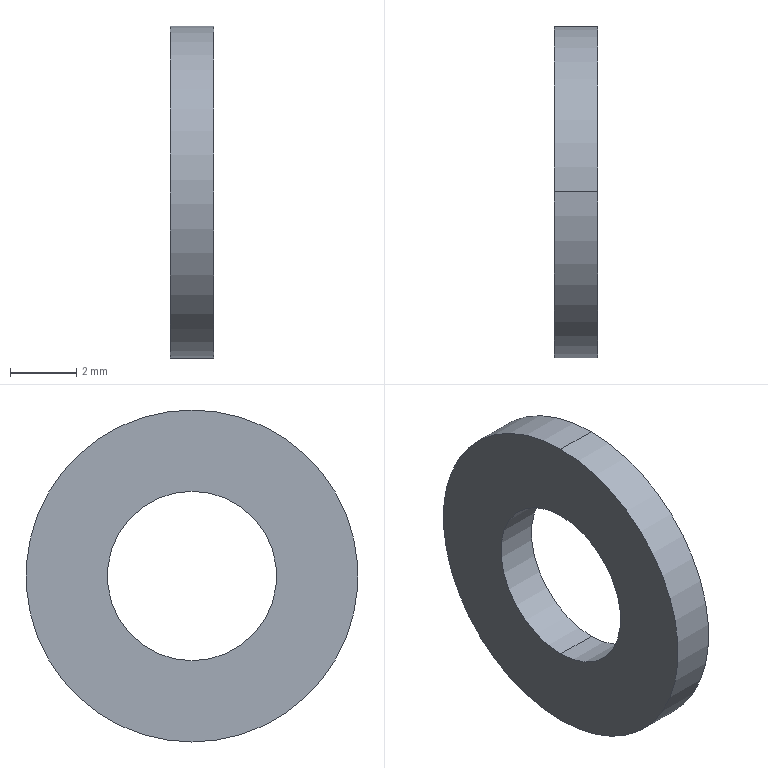Part | STEP file | 0245_Z_041_HCBST5-16_2 | 1 solid | 6 faces | box 1.3 x 10 x 10 mm | volume 75.545 mm3 | cylinder 4 | plane 2 | commonest cylinder face diameters 5.1 x2 10 x2
STEP:
#1=CARTESIAN_POINT('',(0.,0.,0.));
#2=DIRECTION('',(0.,0.,1.));
#3=DIRECTION('',(1.,0.,0.));
#4=AXIS2_PLACEMENT_3D('',#1,#2,#3);
#5=CARTESIAN_POINT('',(4.9,0.,2.55));
#6=VERTEX_POINT('',#5);
#7=CARTESIAN_POINT('',(3.6,0.,2.55));
#8=VERTEX_POINT('',#7);
#9=CARTESIAN_POINT('',(3.6,0.,2.55));
#10=DIRECTION('',(-1.,0.,0.));
#11=VECTOR('',#10,1.);
#12=LINE('',#9,#11);
#13=CARTESIAN_POINT('',(3.6,0.,0.));
#14=DIRECTION('',(-1.,0.,0.));
#15=DIRECTION('',(0.,0.,1.));
#16=AXIS2_PLACEMENT_3D('',#13,#14,#15);
#17=CYLINDRICAL_SURFACE('',#16,2.55);
#18=CARTESIAN_POINT('',(6.283,0.));
#19=DIRECTION('',(0.,1.));
#20=VECTOR('',#19,1.);
#21=LINE('',#18,#20);
#22=(GEOMETRIC_REPRESENTATION_CONTEXT(2)PARAMETRIC_REPRESENTATION_CONTEXT()REPRESENTATION_CONTEXT('',''));
#23=DEFINITIONAL_REPRESENTATION('',(#21),#22);
#24=PCURVE('',#17,#23);
#25=CARTESIAN_POINT('',(3.6,0.,0.));
#26=DIRECTION('',(-1.,0.,0.));
#27=DIRECTION('',(0.,0.,1.));
#28=AXIS2_PLACEMENT_3D('',#25,#26,#27);
#29=CYLINDRICAL_SURFACE('',#28,2.55);
#30=CARTESIAN_POINT('',(0.,0.));
#31=DIRECTION('',(0.,1.));
#32=VECTOR('',#31,1.);
#33=LINE('',#30,#32);
#34=(GEOMETRIC_REPRESENTATION_CONTEXT(2)PARAMETRIC_REPRESENTATION_CONTEXT()REPRESENTATION_CONTEXT('',''));
#35=DEFINITIONAL_REPRESENTATION('',(#33),#34);
#36=PCURVE('',#29,#35);
#37=SURFACE_CURVE('',#12,(#24,#36),.PCURVE_S1.);
#38=EDGE_CURVE('',#6,#8,#37,.T.);
#39=ORIENTED_EDGE('',*,*,#38,.T.);
#40=CARTESIAN_POINT('',(3.6,0.,-2.55));
#41=VERTEX_POINT('',#40);
#42=CARTESIAN_POINT('',(3.6,0.,0.));
#43=DIRECTION('',(1.,0.,0.));
#44=DIRECTION('',(0.,0.,1.));
#45=AXIS2_PLACEMENT_3D('',#42,#43,#44);
#46=CIRCLE('',#45,2.55);
#47=CARTESIAN_POINT('',(6.283,0.));
#48=DIRECTION('',(-1.,0.));
#49=VECTOR('',#48,1.);
#50=LINE('',#47,#49);
#51=(GEOMETRIC_REPRESENTATION_CONTEXT(2)PARAMETRIC_REPRESENTATION_CONTEXT()REPRESENTATION_CONTEXT('',''));
#52=DEFINITIONAL_REPRESENTATION('',(#50),#51);
#53=PCURVE('',#17,#52);
#54=CARTESIAN_POINT('',(3.6,0.,0.));
#55=DIRECTION('',(-1.,0.,0.));
#56=DIRECTION('',(0.,0.,1.));
#57=AXIS2_PLACEMENT_3D('',#54,#55,#56);
#58=PLANE('',#57);
#59=CARTESIAN_POINT('',(2.55,0.));
#60=CARTESIAN_POINT('',(2.55,-4.417));
#61=CARTESIAN_POINT('',(-1.275,-2.208));
#62=CARTESIAN_POINT('',(-5.1,0.));
#63=CARTESIAN_POINT('',(-1.275,2.208));
#64=CARTESIAN_POINT('',(2.55,4.417));
#65=CARTESIAN_POINT('',(2.55,0.));
#66=(BOUNDED_CURVE()B_SPLINE_CURVE(2,(#59,#60,#61,#62,#63,#64,#65),.UNSPECIFIED.,.T.,.F.)B_SPLINE_CURVE_WITH_KNOTS((1,2,2,2,2,1),(-2.094,0.,2.094,4.189,6.283,8.378),.UNSPECIFIED.)CURVE()GEOMETRIC_REPRESENTATION_ITEM()RATIONAL_B_SPLINE_CURVE((1.,0.5,1.,0.5,1.,0.5,1.))REPRESENTATION_ITEM(''));
#67=(GEOMETRIC_REPRESENTATION_CONTEXT(2)PARAMETRIC_REPRESENTATION_CONTEXT()REPRESENTATION_CONTEXT('',''));
#68=DEFINITIONAL_REPRESENTATION('',(#66),#67);
#69=PCURVE('',#58,#68);
#70=SURFACE_CURVE('',#46,(#53,#69),.PCURVE_S1.);
#71=EDGE_CURVE('',#8,#41,#70,.T.);
#72=ORIENTED_EDGE('',*,*,#71,.T.);
#73=CARTESIAN_POINT('',(4.9,0.,-2.55));
#74=VERTEX_POINT('',#73);
#75=CARTESIAN_POINT('',(3.6,0.,-2.55));
#76=DIRECTION('',(-1.,0.,0.));
#77=VECTOR('',#76,1.);
#78=LINE('',#75,#77);
#79=CARTESIAN_POINT('',(3.142,0.));
#80=DIRECTION('',(0.,1.));
#81=VECTOR('',#80,1.);
#82=LINE('',#79,#81);
#83=(GEOMETRIC_REPRESENTATION_CONTEXT(2)PARAMETRIC_REPRESENTATION_CONTEXT()REPRESENTATION_CONTEXT('',''));
#84=DEFINITIONAL_REPRESENTATION('',(#82),#83);
#85=PCURVE('',#17,#84);
#86=CARTESIAN_POINT('',(3.142,0.));
#87=DIRECTION('',(0.,1.));
#88=VECTOR('',#87,1.);
#89=LINE('',#86,#88);
#90=(GEOMETRIC_REPRESENTATION_CONTEXT(2)PARAMETRIC_REPRESENTATION_CONTEXT()REPRESENTATION_CONTEXT('',''));
#91=DEFINITIONAL_REPRESENTATION('',(#89),#90);
#92=PCURVE('',#29,#91);
#93=SURFACE_CURVE('',#78,(#85,#92),.PCURVE_S1.);
#94=EDGE_CURVE('',#74,#41,#93,.T.);
#95=ORIENTED_EDGE('',*,*,#94,.F.);
#96=CARTESIAN_POINT('',(4.9,0.,0.));
#97=DIRECTION('',(1.,0.,0.));
#98=DIRECTION('',(0.,0.,1.));
#99=AXIS2_PLACEMENT_3D('',#96,#97,#98);
#100=CIRCLE('',#99,2.55);
#101=CARTESIAN_POINT('',(6.283,-1.3));
#102=DIRECTION('',(-1.,0.));
#103=VECTOR('',#102,1.);
#104=LINE('',#101,#103);
#105=(GEOMETRIC_REPRESENTATION_CONTEXT(2)PARAMETRIC_REPRESENTATION_CONTEXT()REPRESENTATION_CONTEXT('',''));
#106=DEFINITIONAL_REPRESENTATION('',(#104),#105);
#107=PCURVE('',#17,#106);
#108=CARTESIAN_POINT('',(4.9,0.,0.));
#109=DIRECTION('',(-1.,0.,0.));
#110=DIRECTION('',(0.,0.,1.));
#111=AXIS2_PLACEMENT_3D('',#108,#109,#110);
#112=PLANE('',#111);
#113=CARTESIAN_POINT('',(2.55,0.));
#114=CARTESIAN_POINT('',(2.55,-4.417));
#115=CARTESIAN_POINT('',(-1.275,-2.208));
#116=CARTESIAN_POINT('',(-5.1,0.));
#117=CARTESIAN_POINT('',(-1.275,2.208));
#118=CARTESIAN_POINT('',(2.55,4.417));
#119=CARTESIAN_POINT('',(2.55,0.));
#120=(BOUNDED_CURVE()B_SPLINE_CURVE(2,(#113,#114,#115,#116,#117,#118,#119),.UNSPECIFIED.,.T.,.F.)B_SPLINE_CURVE_WITH_KNOTS((1,2,2,2,2,1),(-2.094,0.,2.094,4.189,6.283,8.378),.UNSPECIFIED.)CURVE()GEOMETRIC_REPRESENTATION_ITEM()RATIONAL_B_SPLINE_CURVE((1.,0.5,1.,0.5,1.,0.5,1.))REPRESENTATION_ITEM(''));
#121=(GEOMETRIC_REPRESENTATION_CONTEXT(2)PARAMETRIC_REPRESENTATION_CONTEXT()REPRESENTATION_CONTEXT('',''));
#122=DEFINITIONAL_REPRESENTATION('',(#120),#121);
#123=PCURVE('',#112,#122);
#124=SURFACE_CURVE('',#100,(#107,#123),.PCURVE_S1.);
#125=EDGE_CURVE('',#6,#74,#124,.T.);
#126=ORIENTED_EDGE('',*,*,#125,.F.);
#127=EDGE_LOOP('',(#39,#72,#95,#126));
#128=FACE_BOUND('',#127,.F.);
#129=ADVANCED_FACE('',(#128),#17,.F.);
#130=CARTESIAN_POINT('',(4.9,0.,5.));
#131=VERTEX_POINT('',#130);
#132=CARTESIAN_POINT('',(4.9,0.,-5.));
#133=VERTEX_POINT('',#132);
#134=CARTESIAN_POINT('',(4.9,0.,0.));
#135=DIRECTION('',(-1.,0.,0.));
#136=DIRECTION('',(0.,0.,1.));
#137=AXIS2_PLACEMENT_3D('',#134,#135,#136);
#138=CIRCLE('',#137,5.);
#139=CARTESIAN_POINT('',(3.6,0.,0.));
#140=DIRECTION('',(-1.,0.,0.));
#141=DIRECTION('',(0.,0.,1.));
#142=AXIS2_PLACEMENT_3D('',#139,#140,#141);
#143=CYLINDRICAL_SURFACE('',#142,5.);
#144=CARTESIAN_POINT('',(0.,-1.3));
#145=DIRECTION('',(1.,0.));
#146=VECTOR('',#145,1.);
#147=LINE('',#144,#146);
#148=(GEOMETRIC_REPRESENTATION_CONTEXT(2)PARAMETRIC_REPRESENTATION_CONTEXT()REPRESENTATION_CONTEXT('',''));
#149=DEFINITIONAL_REPRESENTATION('',(#147),#148);
#150=PCURVE('',#143,#149);
#151=CARTESIAN_POINT('',(0.,0.));
#152=DIRECTION('',(1.,0.));
#153=AXIS2_PLACEMENT_2D('',#151,#152);
#154=CIRCLE('',#153,5.);
#155=(GEOMETRIC_REPRESENTATION_CONTEXT(2)PARAMETRIC_REPRESENTATION_CONTEXT()REPRESENTATION_CONTEXT('',''));
#156=DEFINITIONAL_REPRESENTATION('',(#154),#155);
#157=PCURVE('',#112,#156);
#158=SURFACE_CURVE('',#138,(#150,#157),.PCURVE_S1.);
#159=EDGE_CURVE('',#131,#133,#158,.T.);
#160=ORIENTED_EDGE('',*,*,#159,.T.);
#161=CARTESIAN_POINT('',(3.6,0.,-5.));
#162=VERTEX_POINT('',#161);
#163=CARTESIAN_POINT('',(3.6,0.,-5.));
#164=DIRECTION('',(-1.,0.,0.));
#165=VECTOR('',#164,1.);
#166=LINE('',#163,#165);
#167=CARTESIAN_POINT('',(3.142,0.));
#168=DIRECTION('',(0.,1.));
#169=VECTOR('',#168,1.);
#170=LINE('',#167,#169);
#171=(GEOMETRIC_REPRESENTATION_CONTEXT(2)PARAMETRIC_REPRESENTATION_CONTEXT()REPRESENTATION_CONTEXT('',''));
#172=DEFINITIONAL_REPRESENTATION('',(#170),#171);
#173=PCURVE('',#143,#172);
#174=CARTESIAN_POINT('',(3.6,0.,0.));
#175=DIRECTION('',(-1.,0.,0.));
#176=DIRECTION('',(0.,0.,1.));
#177=AXIS2_PLACEMENT_3D('',#174,#175,#176);
#178=CYLINDRICAL_SURFACE('',#177,5.);
#179=CARTESIAN_POINT('',(3.142,0.));
#180=DIRECTION('',(0.,1.));
#181=VECTOR('',#180,1.);
#182=LINE('',#179,#181);
#183=(GEOMETRIC_REPRESENTATION_CONTEXT(2)PARAMETRIC_REPRESENTATION_CONTEXT()REPRESENTATION_CONTEXT('',''));
#184=DEFINITIONAL_REPRESENTATION('',(#182),#183);
#185=PCURVE('',#178,#184);
#186=SURFACE_CURVE('',#166,(#173,#185),.PCURVE_S1.);
#187=EDGE_CURVE('',#133,#162,#186,.T.);
#188=ORIENTED_EDGE('',*,*,#187,.T.);
#189=CARTESIAN_POINT('',(3.6,0.,5.));
#190=VERTEX_POINT('',#189);
#191=CARTESIAN_POINT('',(3.6,0.,0.));
#192=DIRECTION('',(1.,0.,0.));
#193=DIRECTION('',(0.,0.,1.));
#194=AXIS2_PLACEMENT_3D('',#191,#192,#193);
#195=CIRCLE('',#194,5.);
#196=CARTESIAN_POINT('',(6.283,0.));
#197=DIRECTION('',(-1.,0.));
#198=VECTOR('',#197,1.);
#199=LINE('',#196,#198);
#200=(GEOMETRIC_REPRESENTATION_CONTEXT(2)PARAMETRIC_REPRESENTATION_CONTEXT()REPRESENTATION_CONTEXT('',''));
#201=DEFINITIONAL_REPRESENTATION('',(#199),#200);
#202=PCURVE('',#143,#201);
#203=CARTESIAN_POINT('',(5.,0.));
#204=CARTESIAN_POINT('',(5.,-8.66));
#205=CARTESIAN_POINT('',(-2.5,-4.33));
#206=CARTESIAN_POINT('',(-10.,0.));
#207=CARTESIAN_POINT('',(-2.5,4.33));
#208=CARTESIAN_POINT('',(5.,8.66));
#209=CARTESIAN_POINT('',(5.,0.));
#210=(BOUNDED_CURVE()B_SPLINE_CURVE(2,(#203,#204,#205,#206,#207,#208,#209),.UNSPECIFIED.,.T.,.F.)B_SPLINE_CURVE_WITH_KNOTS((1,2,2,2,2,1),(-2.094,0.,2.094,4.189,6.283,8.378),.UNSPECIFIED.)CURVE()GEOMETRIC_REPRESENTATION_ITEM()RATIONAL_B_SPLINE_CURVE((1.,0.5,1.,0.5,1.,0.5,1.))REPRESENTATION_ITEM(''));
#211=(GEOMETRIC_REPRESENTATION_CONTEXT(2)PARAMETRIC_REPRESENTATION_CONTEXT()REPRESENTATION_CONTEXT('',''));
#212=DEFINITIONAL_REPRESENTATION('',(#210),#211);
#213=PCURVE('',#58,#212);
#214=SURFACE_CURVE('',#195,(#202,#213),.PCURVE_S1.);
#215=EDGE_CURVE('',#162,#190,#214,.T.);
#216=ORIENTED_EDGE('',*,*,#215,.T.);
#217=CARTESIAN_POINT('',(3.6,0.,5.));
#218=DIRECTION('',(-1.,0.,0.));
#219=VECTOR('',#218,1.);
#220=LINE('',#217,#219);
#221=CARTESIAN_POINT('',(0.,0.));
#222=DIRECTION('',(0.,1.));
#223=VECTOR('',#222,1.);
#224=LINE('',#221,#223);
#225=(GEOMETRIC_REPRESENTATION_CONTEXT(2)PARAMETRIC_REPRESENTATION_CONTEXT()REPRESENTATION_CONTEXT('',''));
#226=DEFINITIONAL_REPRESENTATION('',(#224),#225);
#227=PCURVE('',#143,#226);
#228=CARTESIAN_POINT('',(6.283,0.));
#229=DIRECTION('',(0.,1.));
#230=VECTOR('',#229,1.);
#231=LINE('',#228,#230);
#232=(GEOMETRIC_REPRESENTATION_CONTEXT(2)PARAMETRIC_REPRESENTATION_CONTEXT()REPRESENTATION_CONTEXT('',''));
#233=DEFINITIONAL_REPRESENTATION('',(#231),#232);
#234=PCURVE('',#178,#233);
#235=SURFACE_CURVE('',#220,(#227,#234),.PCURVE_S1.);
#236=EDGE_CURVE('',#131,#190,#235,.T.);
#237=ORIENTED_EDGE('',*,*,#236,.F.);
#238=EDGE_LOOP('',(#160,#188,#216,#237));
#239=FACE_BOUND('',#238,.T.);
#240=ADVANCED_FACE('',(#239),#143,.T.);
#241=ORIENTED_EDGE('',*,*,#125,.F.);
#242=CARTESIAN_POINT('',(4.9,0.,0.));
#243=DIRECTION('',(1.,0.,0.));
#244=DIRECTION('',(0.,0.,1.));
#245=AXIS2_PLACEMENT_3D('',#242,#243,#244);
#246=CIRCLE('',#245,2.55);
#247=CARTESIAN_POINT('',(2.55,0.));
#248=CARTESIAN_POINT('',(2.55,-4.417));
#249=CARTESIAN_POINT('',(-1.275,-2.208));
#250=CARTESIAN_POINT('',(-5.1,0.));
#251=CARTESIAN_POINT('',(-1.275,2.208));
#252=CARTESIAN_POINT('',(2.55,4.417));
#253=CARTESIAN_POINT('',(2.55,0.));
#254=(BOUNDED_CURVE()B_SPLINE_CURVE(2,(#247,#248,#249,#250,#251,#252,#253),.UNSPECIFIED.,.T.,.F.)B_SPLINE_CURVE_WITH_KNOTS((1,2,2,2,2,1),(-2.094,0.,2.094,4.189,6.283,8.378),.UNSPECIFIED.)CURVE()GEOMETRIC_REPRESENTATION_ITEM()RATIONAL_B_SPLINE_CURVE((1.,0.5,1.,0.5,1.,0.5,1.))REPRESENTATION_ITEM(''));
#255=(GEOMETRIC_REPRESENTATION_CONTEXT(2)PARAMETRIC_REPRESENTATION_CONTEXT()REPRESENTATION_CONTEXT('',''));
#256=DEFINITIONAL_REPRESENTATION('',(#254),#255);
#257=PCURVE('',#112,#256);
#258=CARTESIAN_POINT('',(6.283,-1.3));
#259=DIRECTION('',(-1.,0.));
#260=VECTOR('',#259,1.);
#261=LINE('',#258,#260);
#262=(GEOMETRIC_REPRESENTATION_CONTEXT(2)PARAMETRIC_REPRESENTATION_CONTEXT()REPRESENTATION_CONTEXT('',''));
#263=DEFINITIONAL_REPRESENTATION('',(#261),#262);
#264=PCURVE('',#29,#263);
#265=SURFACE_CURVE('',#246,(#257,#264),.PCURVE_S1.);
#266=EDGE_CURVE('',#74,#6,#265,.T.);
#267=ORIENTED_EDGE('',*,*,#266,.F.);
#268=EDGE_LOOP('',(#241,#267));
#269=FACE_BOUND('',#268,.T.);
#270=ORIENTED_EDGE('',*,*,#159,.F.);
#271=CARTESIAN_POINT('',(4.9,0.,0.));
#272=DIRECTION('',(-1.,0.,0.));
#273=DIRECTION('',(0.,0.,1.));
#274=AXIS2_PLACEMENT_3D('',#271,#272,#273);
#275=CIRCLE('',#274,5.);
#276=CARTESIAN_POINT('',(0.,0.));
#277=DIRECTION('',(1.,0.));
#278=AXIS2_PLACEMENT_2D('',#276,#277);
#279=CIRCLE('',#278,5.);
#280=(GEOMETRIC_REPRESENTATION_CONTEXT(2)PARAMETRIC_REPRESENTATION_CONTEXT()REPRESENTATION_CONTEXT('',''));
#281=DEFINITIONAL_REPRESENTATION('',(#279),#280);
#282=PCURVE('',#112,#281);
#283=CARTESIAN_POINT('',(0.,-1.3));
#284=DIRECTION('',(1.,0.));
#285=VECTOR('',#284,1.);
#286=LINE('',#283,#285);
#287=(GEOMETRIC_REPRESENTATION_CONTEXT(2)PARAMETRIC_REPRESENTATION_CONTEXT()REPRESENTATION_CONTEXT('',''));
#288=DEFINITIONAL_REPRESENTATION('',(#286),#287);
#289=PCURVE('',#178,#288);
#290=SURFACE_CURVE('',#275,(#282,#289),.PCURVE_S1.);
#291=EDGE_CURVE('',#133,#131,#290,.T.);
#292=ORIENTED_EDGE('',*,*,#291,.F.);
#293=EDGE_LOOP('',(#270,#292));
#294=FACE_BOUND('',#293,.T.);
#295=ADVANCED_FACE('',(#269,#294),#112,.F.);
#296=CARTESIAN_POINT('',(3.6,0.,0.));
#297=DIRECTION('',(1.,0.,0.));
#298=DIRECTION('',(0.,0.,1.));
#299=AXIS2_PLACEMENT_3D('',#296,#297,#298);
#300=CIRCLE('',#299,2.55);
#301=CARTESIAN_POINT('',(6.283,0.));
#302=DIRECTION('',(-1.,0.));
#303=VECTOR('',#302,1.);
#304=LINE('',#301,#303);
#305=(GEOMETRIC_REPRESENTATION_CONTEXT(2)PARAMETRIC_REPRESENTATION_CONTEXT()REPRESENTATION_CONTEXT('',''));
#306=DEFINITIONAL_REPRESENTATION('',(#304),#305);
#307=PCURVE('',#29,#306);
#308=CARTESIAN_POINT('',(2.55,0.));
#309=CARTESIAN_POINT('',(2.55,-4.417));
#310=CARTESIAN_POINT('',(-1.275,-2.208));
#311=CARTESIAN_POINT('',(-5.1,0.));
#312=CARTESIAN_POINT('',(-1.275,2.208));
#313=CARTESIAN_POINT('',(2.55,4.417));
#314=CARTESIAN_POINT('',(2.55,0.));
#315=(BOUNDED_CURVE()B_SPLINE_CURVE(2,(#308,#309,#310,#311,#312,#313,#314),.UNSPECIFIED.,.T.,.F.)B_SPLINE_CURVE_WITH_KNOTS((1,2,2,2,2,1),(-2.094,0.,2.094,4.189,6.283,8.378),.UNSPECIFIED.)CURVE()GEOMETRIC_REPRESENTATION_ITEM()RATIONAL_B_SPLINE_CURVE((1.,0.5,1.,0.5,1.,0.5,1.))REPRESENTATION_ITEM(''));
#316=(GEOMETRIC_REPRESENTATION_CONTEXT(2)PARAMETRIC_REPRESENTATION_CONTEXT()REPRESENTATION_CONTEXT('',''));
#317=DEFINITIONAL_REPRESENTATION('',(#315),#316);
#318=PCURVE('',#58,#317);
#319=SURFACE_CURVE('',#300,(#307,#318),.PCURVE_S1.);
#320=EDGE_CURVE('',#41,#8,#319,.T.);
#321=ORIENTED_EDGE('',*,*,#320,.T.);
#322=ORIENTED_EDGE('',*,*,#38,.F.);
#323=ORIENTED_EDGE('',*,*,#266,.F.);
#324=ORIENTED_EDGE('',*,*,#94,.T.);
#325=EDGE_LOOP('',(#321,#322,#323,#324));
#326=FACE_BOUND('',#325,.F.);
#327=ADVANCED_FACE('',(#326),#29,.F.);
#328=ORIENTED_EDGE('',*,*,#187,.F.);
#329=ORIENTED_EDGE('',*,*,#291,.T.);
#330=ORIENTED_EDGE('',*,*,#236,.T.);
#331=CARTESIAN_POINT('',(3.6,0.,0.));
#332=DIRECTION('',(1.,0.,0.));
#333=DIRECTION('',(0.,0.,1.));
#334=AXIS2_PLACEMENT_3D('',#331,#332,#333);
#335=CIRCLE('',#334,5.);
#336=CARTESIAN_POINT('',(6.283,0.));
#337=DIRECTION('',(-1.,0.));
#338=VECTOR('',#337,1.);
#339=LINE('',#336,#338);
#340=(GEOMETRIC_REPRESENTATION_CONTEXT(2)PARAMETRIC_REPRESENTATION_CONTEXT()REPRESENTATION_CONTEXT('',''));
#341=DEFINITIONAL_REPRESENTATION('',(#339),#340);
#342=PCURVE('',#178,#341);
#343=CARTESIAN_POINT('',(5.,0.));
#344=CARTESIAN_POINT('',(5.,-8.66));
#345=CARTESIAN_POINT('',(-2.5,-4.33));
#346=CARTESIAN_POINT('',(-10.,0.));
#347=CARTESIAN_POINT('',(-2.5,4.33));
#348=CARTESIAN_POINT('',(5.,8.66));
#349=CARTESIAN_POINT('',(5.,0.));
#350=(BOUNDED_CURVE()B_SPLINE_CURVE(2,(#343,#344,#345,#346,#347,#348,#349),.UNSPECIFIED.,.T.,.F.)B_SPLINE_CURVE_WITH_KNOTS((1,2,2,2,2,1),(-2.094,0.,2.094,4.189,6.283,8.378),.UNSPECIFIED.)CURVE()GEOMETRIC_REPRESENTATION_ITEM()RATIONAL_B_SPLINE_CURVE((1.,0.5,1.,0.5,1.,0.5,1.))REPRESENTATION_ITEM(''));
#351=(GEOMETRIC_REPRESENTATION_CONTEXT(2)PARAMETRIC_REPRESENTATION_CONTEXT()REPRESENTATION_CONTEXT('',''));
#352=DEFINITIONAL_REPRESENTATION('',(#350),#351);
#353=PCURVE('',#58,#352);
#354=SURFACE_CURVE('',#335,(#342,#353),.PCURVE_S1.);
#355=EDGE_CURVE('',#190,#162,#354,.T.);
#356=ORIENTED_EDGE('',*,*,#355,.T.);
#357=EDGE_LOOP('',(#328,#329,#330,#356));
#358=FACE_BOUND('',#357,.T.);
#359=ADVANCED_FACE('',(#358),#178,.T.);
#360=ORIENTED_EDGE('',*,*,#71,.T.);
#361=ORIENTED_EDGE('',*,*,#320,.T.);
#362=EDGE_LOOP('',(#360,#361));
#363=FACE_BOUND('',#362,.T.);
#364=ORIENTED_EDGE('',*,*,#355,.F.);
#365=ORIENTED_EDGE('',*,*,#215,.F.);
#366=EDGE_LOOP('',(#364,#365));
#367=FACE_BOUND('',#366,.T.);
#368=ADVANCED_FACE('',(#363,#367),#58,.T.);
#369=CLOSED_SHELL('',(#129,#240,#295,#327,#359,#368));
#370=MANIFOLD_SOLID_BREP('',#369);
#371=(LENGTH_UNIT()NAMED_UNIT(*)SI_UNIT(.MILLI.,.METRE.));
#372=UNCERTAINTY_MEASURE_WITH_UNIT(LENGTH_MEASURE(0.0000001),#371,'','');
#373=(NAMED_UNIT(*)PLANE_ANGLE_UNIT()SI_UNIT($,.RADIAN.));
#374=(NAMED_UNIT(*)SI_UNIT($,.STERADIAN.)SOLID_ANGLE_UNIT());
#375=(GEOMETRIC_REPRESENTATION_CONTEXT(3)GLOBAL_UNCERTAINTY_ASSIGNED_CONTEXT((#372))GLOBAL_UNIT_ASSIGNED_CONTEXT((#371,#373,#374))REPRESENTATION_CONTEXT('',''));
#376=ADVANCED_BREP_SHAPE_REPRESENTATION('',(#4,#370),#375);